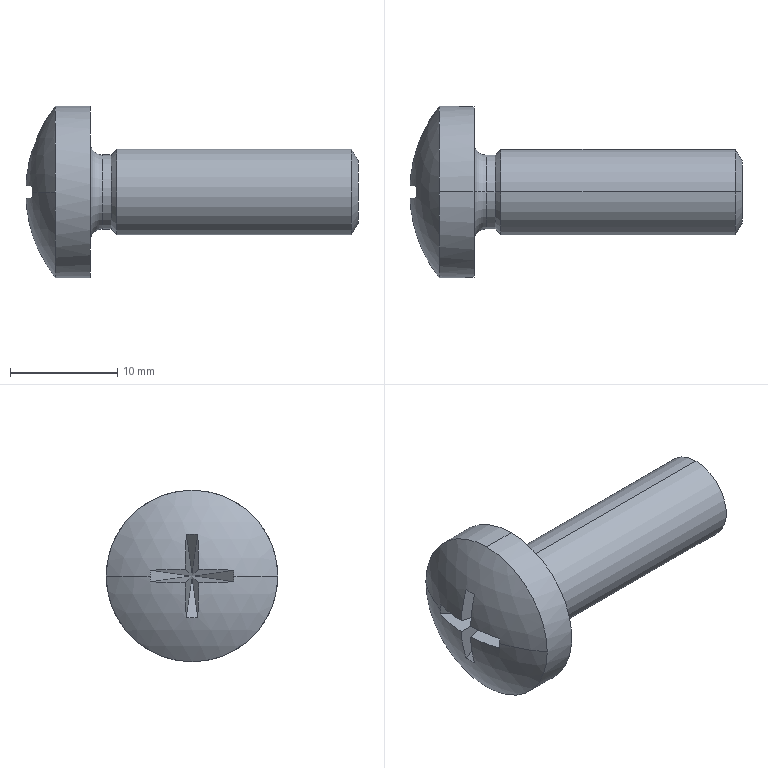Part | SolidWorks | features BlendCut 1, LPattern 1, MirrorPattern 1, RevCut 1, Revolution 1 | 1 solid | 28 faces | box 30.97 x 16 x 16 mm | volume 2140 mm3 | plane 14 | cylinder 6 | cone 4 | torus 2 | sphere 2 | commonest cylinder face diameters 6.928 x2 8 x2 16 x2
STEP:
#1=CARTESIAN_POINT('',(31.,0.,2.918));
#2=VERTEX_POINT('',#1);
#3=CARTESIAN_POINT('',(31.,0.,-2.918));
#4=VERTEX_POINT('',#3);
#5=CARTESIAN_POINT('',(31.,0.,0.));
#6=DIRECTION('',(-1.,0.,0.));
#7=DIRECTION('',(0.,0.,1.));
#8=AXIS2_PLACEMENT_3D('',#5,#6,#7);
#9=CIRCLE('',#8,2.918);
#10=EDGE_CURVE('',#2,#4,#9,.T.);
#11=ORIENTED_EDGE('',*,*,#10,.T.);
#12=CARTESIAN_POINT('',(30.382,0.,-4.));
#13=VERTEX_POINT('',#12);
#14=CARTESIAN_POINT('',(30.382,0.,-4.));
#15=DIRECTION('',(-0.4959,0.,-0.8684));
#16=VECTOR('',#15,1000.);
#17=LINE('',#14,#16);
#18=EDGE_CURVE('',#4,#13,#17,.T.);
#19=ORIENTED_EDGE('',*,*,#18,.T.);
#20=CARTESIAN_POINT('',(30.382,0.,4.));
#21=VERTEX_POINT('',#20);
#22=CARTESIAN_POINT('',(30.382,0.,0.));
#23=DIRECTION('',(-1.,0.,0.));
#24=DIRECTION('',(0.,0.,1.));
#25=AXIS2_PLACEMENT_3D('',#22,#23,#24);
#26=CIRCLE('',#25,4.);
#27=EDGE_CURVE('',#21,#13,#26,.T.);
#28=ORIENTED_EDGE('',*,*,#27,.F.);
#29=CARTESIAN_POINT('',(30.382,0.,4.));
#30=DIRECTION('',(-0.4959,0.,0.8684));
#31=VECTOR('',#30,1000.);
#32=LINE('',#29,#31);
#33=EDGE_CURVE('',#2,#21,#32,.T.);
#34=ORIENTED_EDGE('',*,*,#33,.F.);
#35=EDGE_LOOP('',(#11,#19,#28,#34));
#36=FACE_OUTER_BOUND('',#35,.T.);
#37=CARTESIAN_POINT('',(30.382,0.,0.));
#38=DIRECTION('',(-1.,0.,0.));
#39=DIRECTION('',(0.,0.,1.));
#40=AXIS2_PLACEMENT_3D('',#37,#38,#39);
#41=CONICAL_SURFACE('',#40,4.,1.052);
#42=ADVANCED_FACE('',(#36),#41,.T.);
#43=CARTESIAN_POINT('',(7.964,0.,3.464));
#44=VERTEX_POINT('',#43);
#45=CARTESIAN_POINT('',(7.964,0.,-3.464));
#46=VERTEX_POINT('',#45);
#47=CARTESIAN_POINT('',(7.964,0.,0.));
#48=DIRECTION('',(-1.,0.,0.));
#49=DIRECTION('',(0.,0.,1.));
#50=AXIS2_PLACEMENT_3D('',#47,#48,#49);
#51=CIRCLE('',#50,3.464);
#52=EDGE_CURVE('',#44,#46,#51,.T.);
#53=ORIENTED_EDGE('',*,*,#52,.F.);
#54=CARTESIAN_POINT('',(8.5,0.,4.));
#55=VERTEX_POINT('',#54);
#56=CARTESIAN_POINT('',(8.5,0.,4.));
#57=DIRECTION('',(0.7071,0.,0.7071));
#58=VECTOR('',#57,1000.);
#59=LINE('',#56,#58);
#60=EDGE_CURVE('',#44,#55,#59,.T.);
#61=ORIENTED_EDGE('',*,*,#60,.T.);
#62=CARTESIAN_POINT('',(8.5,0.,-4.));
#63=VERTEX_POINT('',#62);
#64=CARTESIAN_POINT('',(8.5,0.,0.));
#65=DIRECTION('',(-1.,0.,0.));
#66=DIRECTION('',(0.,0.,1.));
#67=AXIS2_PLACEMENT_3D('',#64,#65,#66);
#68=CIRCLE('',#67,4.);
#69=EDGE_CURVE('',#55,#63,#68,.T.);
#70=ORIENTED_EDGE('',*,*,#69,.T.);
#71=CARTESIAN_POINT('',(8.5,0.,-4.));
#72=DIRECTION('',(0.7071,0.,-0.7071));
#73=VECTOR('',#72,1000.);
#74=LINE('',#71,#73);
#75=EDGE_CURVE('',#46,#63,#74,.T.);
#76=ORIENTED_EDGE('',*,*,#75,.F.);
#77=EDGE_LOOP('',(#53,#61,#70,#76));
#78=FACE_OUTER_BOUND('',#77,.T.);
#79=CARTESIAN_POINT('',(8.5,0.,0.));
#80=DIRECTION('',(1.,0.,0.));
#81=DIRECTION('',(0.,0.,-1.));
#82=AXIS2_PLACEMENT_3D('',#79,#80,#81);
#83=CONICAL_SURFACE('',#82,4.,0.7854);
#84=ADVANCED_FACE('',(#78),#83,.T.);
#85=ORIENTED_EDGE('',*,*,#52,.T.);
#86=CARTESIAN_POINT('',(7.136,0.,-3.464));
#87=VERTEX_POINT('',#86);
#88=CARTESIAN_POINT('',(-1.332,0.,-3.464));
#89=DIRECTION('',(-1.,0.,0.));
#90=VECTOR('',#89,1000.);
#91=LINE('',#88,#90);
#92=EDGE_CURVE('',#46,#87,#91,.T.);
#93=ORIENTED_EDGE('',*,*,#92,.T.);
#94=CARTESIAN_POINT('',(7.136,0.,3.464));
#95=VERTEX_POINT('',#94);
#96=CARTESIAN_POINT('',(7.136,0.,0.));
#97=DIRECTION('',(-1.,0.,0.));
#98=DIRECTION('',(0.,0.,1.));
#99=AXIS2_PLACEMENT_3D('',#96,#97,#98);
#100=CIRCLE('',#99,3.464);
#101=EDGE_CURVE('',#95,#87,#100,.T.);
#102=ORIENTED_EDGE('',*,*,#101,.F.);
#103=CARTESIAN_POINT('',(-1.332,0.,3.464));
#104=DIRECTION('',(-1.,0.,0.));
#105=VECTOR('',#104,1000.);
#106=LINE('',#103,#105);
#107=EDGE_CURVE('',#44,#95,#106,.T.);
#108=ORIENTED_EDGE('',*,*,#107,.F.);
#109=EDGE_LOOP('',(#85,#93,#102,#108));
#110=FACE_OUTER_BOUND('',#109,.T.);
#111=CARTESIAN_POINT('',(-1.332,0.,0.));
#112=DIRECTION('',(-1.,0.,0.));
#113=DIRECTION('',(0.,0.,1.));
#114=AXIS2_PLACEMENT_3D('',#111,#112,#113);
#115=CYLINDRICAL_SURFACE('',#114,3.464);
#116=ADVANCED_FACE('',(#110),#115,.T.);
#117=CARTESIAN_POINT('',(6.,0.,-4.6));
#118=VERTEX_POINT('',#117);
#119=CARTESIAN_POINT('',(6.,0.,4.6));
#120=VERTEX_POINT('',#119);
#121=CARTESIAN_POINT('',(6.,0.,0.));
#122=DIRECTION('',(-1.,0.,0.));
#123=DIRECTION('',(0.,0.,1.));
#124=AXIS2_PLACEMENT_3D('',#121,#122,#123);
#125=CIRCLE('',#124,4.6);
#126=EDGE_CURVE('',#118,#120,#125,.T.);
#127=ORIENTED_EDGE('',*,*,#126,.F.);
#128=CARTESIAN_POINT('',(7.136,0.,-4.6));
#129=DIRECTION('',(0.,1.,0.));
#130=DIRECTION('',(0.,0.,1.));
#131=AXIS2_PLACEMENT_3D('',#128,#129,#130);
#132=CIRCLE('',#131,1.136);
#133=EDGE_CURVE('',#118,#87,#132,.T.);
#134=ORIENTED_EDGE('',*,*,#133,.T.);
#135=CARTESIAN_POINT('',(7.136,0.,0.));
#136=DIRECTION('',(-1.,0.,0.));
#137=DIRECTION('',(0.,0.,1.));
#138=AXIS2_PLACEMENT_3D('',#135,#136,#137);
#139=CIRCLE('',#138,3.464);
#140=EDGE_CURVE('',#87,#95,#139,.T.);
#141=ORIENTED_EDGE('',*,*,#140,.T.);
#142=CARTESIAN_POINT('',(7.136,0.,4.6));
#143=DIRECTION('',(0.,-1.,0.));
#144=DIRECTION('',(0.,0.,-1.));
#145=AXIS2_PLACEMENT_3D('',#142,#143,#144);
#146=CIRCLE('',#145,1.136);
#147=EDGE_CURVE('',#120,#95,#146,.T.);
#148=ORIENTED_EDGE('',*,*,#147,.F.);
#149=EDGE_LOOP('',(#127,#134,#141,#148));
#150=FACE_OUTER_BOUND('',#149,.T.);
#151=CARTESIAN_POINT('',(7.136,0.,0.));
#152=DIRECTION('',(-1.,0.,0.));
#153=DIRECTION('',(0.,0.,1.));
#154=AXIS2_PLACEMENT_3D('',#151,#152,#153);
#155=TOROIDAL_SURFACE('',#154,4.6,1.136);
#156=ADVANCED_FACE('',(#150),#155,.F.);
#157=CARTESIAN_POINT('',(6.,0.,8.));
#158=VERTEX_POINT('',#157);
#159=CARTESIAN_POINT('',(6.,0.,-8.));
#160=VERTEX_POINT('',#159);
#161=CARTESIAN_POINT('',(6.,0.,0.));
#162=DIRECTION('',(-1.,0.,0.));
#163=DIRECTION('',(0.,0.,1.));
#164=AXIS2_PLACEMENT_3D('',#161,#162,#163);
#165=CIRCLE('',#164,8.);
#166=EDGE_CURVE('',#158,#160,#165,.T.);
#167=ORIENTED_EDGE('',*,*,#166,.T.);
#168=CARTESIAN_POINT('',(2.753,0.,-8.));
#169=VERTEX_POINT('',#168);
#170=CARTESIAN_POINT('',(-1.332,0.,-8.));
#171=DIRECTION('',(-1.,0.,0.));
#172=VECTOR('',#171,1000.);
#173=LINE('',#170,#172);
#174=EDGE_CURVE('',#160,#169,#173,.T.);
#175=ORIENTED_EDGE('',*,*,#174,.T.);
#176=CARTESIAN_POINT('',(2.753,8.,0.));
#177=VERTEX_POINT('',#176);
#178=CARTESIAN_POINT('',(2.753,0.,0.));
#179=DIRECTION('',(-1.,0.,0.));
#180=DIRECTION('',(0.,0.,1.));
#181=AXIS2_PLACEMENT_3D('',#178,#179,#180);
#182=CIRCLE('',#181,8.);
#183=EDGE_CURVE('',#177,#169,#182,.T.);
#184=ORIENTED_EDGE('',*,*,#183,.F.);
#185=CARTESIAN_POINT('',(2.753,0.,8.));
#186=VERTEX_POINT('',#185);
#187=CARTESIAN_POINT('',(2.753,0.,0.));
#188=DIRECTION('',(-1.,0.,0.));
#189=DIRECTION('',(0.,0.,1.));
#190=AXIS2_PLACEMENT_3D('',#187,#188,#189);
#191=CIRCLE('',#190,8.);
#192=EDGE_CURVE('',#186,#177,#191,.T.);
#193=ORIENTED_EDGE('',*,*,#192,.F.);
#194=CARTESIAN_POINT('',(-1.332,0.,8.));
#195=DIRECTION('',(-1.,0.,0.));
#196=VECTOR('',#195,1000.);
#197=LINE('',#194,#196);
#198=EDGE_CURVE('',#158,#186,#197,.T.);
#199=ORIENTED_EDGE('',*,*,#198,.F.);
#200=EDGE_LOOP('',(#167,#175,#184,#193,#199));
#201=FACE_OUTER_BOUND('',#200,.T.);
#202=CARTESIAN_POINT('',(-1.332,0.,0.));
#203=DIRECTION('',(-1.,0.,0.));
#204=DIRECTION('',(0.,0.,1.));
#205=AXIS2_PLACEMENT_3D('',#202,#203,#204);
#206=CYLINDRICAL_SURFACE('',#205,8.);
#207=ADVANCED_FACE('',(#201),#206,.T.);
#208=ORIENTED_EDGE('',*,*,#183,.T.);
#209=CARTESIAN_POINT('',(2.753,-8.,0.));
#210=VERTEX_POINT('',#209);
#211=CARTESIAN_POINT('',(2.753,0.,0.));
#212=DIRECTION('',(-1.,0.,0.));
#213=DIRECTION('',(0.,0.,1.));
#214=AXIS2_PLACEMENT_3D('',#211,#212,#213);
#215=CIRCLE('',#214,8.);
#216=EDGE_CURVE('',#169,#210,#215,.T.);
#217=ORIENTED_EDGE('',*,*,#216,.T.);
#218=CARTESIAN_POINT('',(0.6022,-3.911,0.));
#219=VERTEX_POINT('',#218);
#220=CARTESIAN_POINT('',(13.,0.,0.));
#221=DIRECTION('',(0.,0.,-1.));
#222=DIRECTION('',(0.,1.,0.));
#223=AXIS2_PLACEMENT_3D('',#220,#221,#222);
#224=CIRCLE('',#223,13.);
#225=EDGE_CURVE('',#210,#219,#224,.T.);
#226=ORIENTED_EDGE('',*,*,#225,.T.);
#227=CARTESIAN_POINT('',(0.6113,-3.902,-0.5419));
#228=VERTEX_POINT('',#227);
#229=CARTESIAN_POINT('',(8.892,4.199,0.));
#230=DIRECTION('',(0.6993,-0.7148,0.));
#231=DIRECTION('',(0.7148,0.6993,0.));
#232=AXIS2_PLACEMENT_3D('',#229,#230,#231);
#233=CIRCLE('',#232,11.597);
#234=EDGE_CURVE('',#219,#228,#233,.T.);
#235=ORIENTED_EDGE('',*,*,#234,.T.);
#236=CARTESIAN_POINT('',(0.0297,-0.621,-0.621));
#237=VERTEX_POINT('',#236);
#238=CARTESIAN_POINT('',(12.848,0.,1.121));
#239=DIRECTION('',(0.1346,0.,-0.9909));
#240=DIRECTION('',(-0.9909,0.,-0.1346));
#241=AXIS2_PLACEMENT_3D('',#238,#239,#240);
#242=CIRCLE('',#241,12.951);
#243=EDGE_CURVE('',#228,#237,#242,.T.);
#244=ORIENTED_EDGE('',*,*,#243,.T.);
#245=CARTESIAN_POINT('',(0.6113,-0.5419,-3.902));
#246=VERTEX_POINT('',#245);
#247=CARTESIAN_POINT('',(12.848,1.121,0.));
#248=DIRECTION('',(0.1346,-0.9909,0.));
#249=DIRECTION('',(0.9909,0.1346,0.));
#250=AXIS2_PLACEMENT_3D('',#247,#248,#249);
#251=CIRCLE('',#250,12.951);
#252=EDGE_CURVE('',#237,#246,#251,.T.);
#253=ORIENTED_EDGE('',*,*,#252,.T.);
#254=CARTESIAN_POINT('',(0.6113,0.5419,-3.902));
#255=VERTEX_POINT('',#254);
#256=CARTESIAN_POINT('',(8.892,0.,4.199));
#257=DIRECTION('',(0.6993,0.,-0.7148));
#258=DIRECTION('',(-0.7148,0.,-0.6993));
#259=AXIS2_PLACEMENT_3D('',#256,#257,#258);
#260=CIRCLE('',#259,11.597);
#261=EDGE_CURVE('',#246,#255,#260,.T.);
#262=ORIENTED_EDGE('',*,*,#261,.T.);
#263=CARTESIAN_POINT('',(0.0297,0.621,-0.621));
#264=VERTEX_POINT('',#263);
#265=CARTESIAN_POINT('',(12.848,-1.121,0.));
#266=DIRECTION('',(0.1346,0.9909,0.));
#267=DIRECTION('',(-0.9909,0.1346,0.));
#268=AXIS2_PLACEMENT_3D('',#265,#266,#267);
#269=CIRCLE('',#268,12.951);
#270=EDGE_CURVE('',#255,#264,#269,.T.);
#271=ORIENTED_EDGE('',*,*,#270,.T.);
#272=CARTESIAN_POINT('',(0.6113,3.902,-0.5419));
#273=VERTEX_POINT('',#272);
#274=CARTESIAN_POINT('',(12.848,0.,1.121));
#275=DIRECTION('',(0.1346,0.,-0.9909));
#276=DIRECTION('',(-0.9909,0.,-0.1346));
#277=AXIS2_PLACEMENT_3D('',#274,#275,#276);
#278=CIRCLE('',#277,12.951);
#279=EDGE_CURVE('',#264,#273,#278,.T.);
#280=ORIENTED_EDGE('',*,*,#279,.T.);
#281=CARTESIAN_POINT('',(0.6022,3.911,0.));
#282=VERTEX_POINT('',#281);
#283=CARTESIAN_POINT('',(8.892,-4.199,0.));
#284=DIRECTION('',(0.6993,0.7148,0.));
#285=DIRECTION('',(-0.7148,0.6993,0.));
#286=AXIS2_PLACEMENT_3D('',#283,#284,#285);
#287=CIRCLE('',#286,11.597);
#288=EDGE_CURVE('',#273,#282,#287,.T.);
#289=ORIENTED_EDGE('',*,*,#288,.T.);
#290=CARTESIAN_POINT('',(13.,0.,0.));
#291=DIRECTION('',(0.,0.,1.));
#292=DIRECTION('',(1.,0.,0.));
#293=AXIS2_PLACEMENT_3D('',#290,#291,#292);
#294=CIRCLE('',#293,13.);
#295=EDGE_CURVE('',#177,#282,#294,.T.);
#296=ORIENTED_EDGE('',*,*,#295,.F.);
#297=EDGE_LOOP('',(#208,#217,#226,#235,#244,#253,#262,#271,#280,#289,#296));
#298=FACE_OUTER_BOUND('',#297,.T.);
#299=CARTESIAN_POINT('',(13.,0.,0.));
#300=DIRECTION('',(0.,0.,-1.));
#301=DIRECTION('',(0.,1.,0.));
#302=AXIS2_PLACEMENT_3D('',#299,#300,#301);
#303=SPHERICAL_SURFACE('',#302,13.);
#304=ADVANCED_FACE('',(#298),#303,.T.);
#305=ORIENTED_EDGE('',*,*,#27,.T.);
#306=CARTESIAN_POINT('',(-1.332,0.,-4.));
#307=DIRECTION('',(-1.,0.,0.));
#308=VECTOR('',#307,1000.);
#309=LINE('',#306,#308);
#310=EDGE_CURVE('',#13,#63,#309,.T.);
#311=ORIENTED_EDGE('',*,*,#310,.T.);
#312=ORIENTED_EDGE('',*,*,#69,.F.);
#313=CARTESIAN_POINT('',(-1.332,0.,4.));
#314=DIRECTION('',(-1.,0.,0.));
#315=VECTOR('',#314,1000.);
#316=LINE('',#313,#315);
#317=EDGE_CURVE('',#21,#55,#316,.T.);
#318=ORIENTED_EDGE('',*,*,#317,.F.);
#319=EDGE_LOOP('',(#305,#311,#312,#318));
#320=FACE_OUTER_BOUND('',#319,.T.);
#321=CARTESIAN_POINT('',(-1.332,0.,0.));
#322=DIRECTION('',(-1.,0.,0.));
#323=DIRECTION('',(0.,0.,1.));
#324=AXIS2_PLACEMENT_3D('',#321,#322,#323);
#325=CYLINDRICAL_SURFACE('',#324,4.);
#326=ADVANCED_FACE('',(#320),#325,.T.);
#327=CARTESIAN_POINT('',(4.6,0.,0.));
#328=VERTEX_POINT('',#327);
#329=CARTESIAN_POINT('',(4.6,0.,0.));
#330=DIRECTION('',(-0.7115,-0.696,-0.09667));
#331=VECTOR('',#330,1000.);
#332=LINE('',#329,#331);
#333=EDGE_CURVE('',#328,#228,#332,.T.);
#334=ORIENTED_EDGE('',*,*,#333,.F.);
#335=CARTESIAN_POINT('',(4.6,0.,0.));
#336=DIRECTION('',(-0.982,-0.1334,-0.1334));
#337=VECTOR('',#336,1000.);
#338=LINE('',#335,#337);
#339=EDGE_CURVE('',#328,#237,#338,.T.);
#340=ORIENTED_EDGE('',*,*,#339,.T.);
#341=ORIENTED_EDGE('',*,*,#243,.F.);
#342=EDGE_LOOP('',(#334,#340,#341));
#343=FACE_OUTER_BOUND('',#342,.T.);
#344=CARTESIAN_POINT('',(4.6,0.,0.));
#345=DIRECTION('',(0.1346,0.,-0.9909));
#346=DIRECTION('',(-0.9909,0.,-0.1346));
#347=AXIS2_PLACEMENT_3D('',#344,#345,#346);
#348=PLANE('',#347);
#349=ADVANCED_FACE('',(#343),#348,.F.);
#350=CARTESIAN_POINT('',(0.0297,-0.621,0.621));
#351=VERTEX_POINT('',#350);
#352=CARTESIAN_POINT('',(0.6113,-3.902,0.5419));
#353=VERTEX_POINT('',#352);
#354=CARTESIAN_POINT('',(12.848,0.,-1.121));
#355=DIRECTION('',(0.1346,0.,0.9909));
#356=DIRECTION('',(0.9909,0.,-0.1346));
#357=AXIS2_PLACEMENT_3D('',#354,#355,#356);
#358=CIRCLE('',#357,12.951);
#359=EDGE_CURVE('',#351,#353,#358,.T.);
#360=ORIENTED_EDGE('',*,*,#359,.F.);
#361=CARTESIAN_POINT('',(4.6,0.,0.));
#362=DIRECTION('',(0.982,0.1334,-0.1334));
#363=VECTOR('',#362,1000.);
#364=LINE('',#361,#363);
#365=EDGE_CURVE('',#351,#328,#364,.T.);
#366=ORIENTED_EDGE('',*,*,#365,.T.);
#367=CARTESIAN_POINT('',(4.6,0.,0.));
#368=DIRECTION('',(-0.7115,-0.696,0.09667));
#369=VECTOR('',#368,1000.);
#370=LINE('',#367,#369);
#371=EDGE_CURVE('',#328,#353,#370,.T.);
#372=ORIENTED_EDGE('',*,*,#371,.T.);
#373=EDGE_LOOP('',(#360,#366,#372));
#374=FACE_OUTER_BOUND('',#373,.T.);
#375=CARTESIAN_POINT('',(4.6,0.,0.));
#376=DIRECTION('',(0.1346,0.,0.9909));
#377=DIRECTION('',(0.9909,0.,-0.1346));
#378=AXIS2_PLACEMENT_3D('',#375,#376,#377);
#379=PLANE('',#378);
#380=ADVANCED_FACE('',(#374),#379,.F.);
#381=ORIENTED_EDGE('',*,*,#310,.F.);
#382=CARTESIAN_POINT('',(30.382,0.,0.));
#383=DIRECTION('',(-1.,0.,0.));
#384=DIRECTION('',(0.,0.,1.));
#385=AXIS2_PLACEMENT_3D('',#382,#383,#384);
#386=CIRCLE('',#385,4.);
#387=EDGE_CURVE('',#13,#21,#386,.T.);
#388=ORIENTED_EDGE('',*,*,#387,.T.);
#389=ORIENTED_EDGE('',*,*,#317,.T.);
#390=CARTESIAN_POINT('',(8.5,0.,0.));
#391=DIRECTION('',(-1.,0.,0.));
#392=DIRECTION('',(0.,0.,1.));
#393=AXIS2_PLACEMENT_3D('',#390,#391,#392);
#394=CIRCLE('',#393,4.);
#395=EDGE_CURVE('',#63,#55,#394,.T.);
#396=ORIENTED_EDGE('',*,*,#395,.F.);
#397=EDGE_LOOP('',(#381,#388,#389,#396));
#398=FACE_OUTER_BOUND('',#397,.T.);
#399=CARTESIAN_POINT('',(-1.332,0.,0.));
#400=DIRECTION('',(-1.,0.,0.));
#401=DIRECTION('',(0.,0.,1.));
#402=AXIS2_PLACEMENT_3D('',#399,#400,#401);
#403=CYLINDRICAL_SURFACE('',#402,4.);
#404=ADVANCED_FACE('',(#398),#403,.T.);
#405=ORIENTED_EDGE('',*,*,#225,.F.);
#406=CARTESIAN_POINT('',(2.753,0.,0.));
#407=DIRECTION('',(-1.,0.,0.));
#408=DIRECTION('',(0.,0.,1.));
#409=AXIS2_PLACEMENT_3D('',#406,#407,#408);
#410=CIRCLE('',#409,8.);
#411=EDGE_CURVE('',#210,#186,#410,.T.);
#412=ORIENTED_EDGE('',*,*,#411,.T.);
#413=ORIENTED_EDGE('',*,*,#192,.T.);
#414=ORIENTED_EDGE('',*,*,#295,.T.);
#415=CARTESIAN_POINT('',(0.6113,3.902,0.5419));
#416=VERTEX_POINT('',#415);
#417=CARTESIAN_POINT('',(8.892,-4.199,0.));
#418=DIRECTION('',(0.6993,0.7148,0.));
#419=DIRECTION('',(-0.7148,0.6993,0.));
#420=AXIS2_PLACEMENT_3D('',#417,#418,#419);
#421=CIRCLE('',#420,11.597);
#422=EDGE_CURVE('',#282,#416,#421,.T.);
#423=ORIENTED_EDGE('',*,*,#422,.T.);
#424=CARTESIAN_POINT('',(0.0297,0.621,0.621));
#425=VERTEX_POINT('',#424);
#426=CARTESIAN_POINT('',(12.848,0.,-1.121));
#427=DIRECTION('',(0.1346,0.,0.9909));
#428=DIRECTION('',(0.9909,0.,-0.1346));
#429=AXIS2_PLACEMENT_3D('',#426,#427,#428);
#430=CIRCLE('',#429,12.951);
#431=EDGE_CURVE('',#416,#425,#430,.T.);
#432=ORIENTED_EDGE('',*,*,#431,.T.);
#433=CARTESIAN_POINT('',(0.6113,0.5419,3.902));
#434=VERTEX_POINT('',#433);
#435=CARTESIAN_POINT('',(12.848,-1.121,0.));
#436=DIRECTION('',(0.1346,0.9909,0.));
#437=DIRECTION('',(-0.9909,0.1346,0.));
#438=AXIS2_PLACEMENT_3D('',#435,#436,#437);
#439=CIRCLE('',#438,12.951);
#440=EDGE_CURVE('',#425,#434,#439,.T.);
#441=ORIENTED_EDGE('',*,*,#440,.T.);
#442=CARTESIAN_POINT('',(0.6113,-0.5419,3.902));
#443=VERTEX_POINT('',#442);
#444=CARTESIAN_POINT('',(8.892,0.,-4.199));
#445=DIRECTION('',(0.6993,0.,0.7148));
#446=DIRECTION('',(0.7148,0.,-0.6993));
#447=AXIS2_PLACEMENT_3D('',#444,#445,#446);
#448=CIRCLE('',#447,11.597);
#449=EDGE_CURVE('',#434,#443,#448,.T.);
#450=ORIENTED_EDGE('',*,*,#449,.T.);
#451=CARTESIAN_POINT('',(12.848,1.121,0.));
#452=DIRECTION('',(0.1346,-0.9909,0.));
#453=DIRECTION('',(0.9909,0.1346,0.));
#454=AXIS2_PLACEMENT_3D('',#451,#452,#453);
#455=CIRCLE('',#454,12.951);
#456=EDGE_CURVE('',#443,#351,#455,.T.);
#457=ORIENTED_EDGE('',*,*,#456,.T.);
#458=ORIENTED_EDGE('',*,*,#359,.T.);
#459=CARTESIAN_POINT('',(8.892,4.199,0.));
#460=DIRECTION('',(0.6993,-0.7148,0.));
#461=DIRECTION('',(0.7148,0.6993,0.));
#462=AXIS2_PLACEMENT_3D('',#459,#460,#461);
#463=CIRCLE('',#462,11.597);
#464=EDGE_CURVE('',#353,#219,#463,.T.);
#465=ORIENTED_EDGE('',*,*,#464,.T.);
#466=EDGE_LOOP('',(#405,#412,#413,#414,#423,#432,#441,#450,#457,#458,#465));
#467=FACE_OUTER_BOUND('',#466,.T.);
#468=CARTESIAN_POINT('',(13.,0.,0.));
#469=DIRECTION('',(0.,0.,-1.));
#470=DIRECTION('',(0.,1.,0.));
#471=AXIS2_PLACEMENT_3D('',#468,#469,#470);
#472=SPHERICAL_SURFACE('',#471,13.);
#473=ADVANCED_FACE('',(#467),#472,.T.);
#474=ORIENTED_EDGE('',*,*,#174,.F.);
#475=CARTESIAN_POINT('',(6.,0.,0.));
#476=DIRECTION('',(-1.,0.,0.));
#477=DIRECTION('',(0.,0.,1.));
#478=AXIS2_PLACEMENT_3D('',#475,#476,#477);
#479=CIRCLE('',#478,8.);
#480=EDGE_CURVE('',#160,#158,#479,.T.);
#481=ORIENTED_EDGE('',*,*,#480,.T.);
#482=ORIENTED_EDGE('',*,*,#198,.T.);
#483=ORIENTED_EDGE('',*,*,#411,.F.);
#484=ORIENTED_EDGE('',*,*,#216,.F.);
#485=EDGE_LOOP('',(#474,#481,#482,#483,#484));
#486=FACE_OUTER_BOUND('',#485,.T.);
#487=CARTESIAN_POINT('',(-1.332,0.,0.));
#488=DIRECTION('',(-1.,0.,0.));
#489=DIRECTION('',(0.,0.,1.));
#490=AXIS2_PLACEMENT_3D('',#487,#488,#489);
#491=CYLINDRICAL_SURFACE('',#490,8.);
#492=ADVANCED_FACE('',(#486),#491,.T.);
#493=ORIENTED_EDGE('',*,*,#166,.F.);
#494=ORIENTED_EDGE('',*,*,#480,.F.);
#495=EDGE_LOOP('',(#493,#494));
#496=FACE_OUTER_BOUND('',#495,.T.);
#497=CARTESIAN_POINT('',(6.,0.,0.));
#498=DIRECTION('',(-1.,0.,0.));
#499=DIRECTION('',(0.,0.,1.));
#500=AXIS2_PLACEMENT_3D('',#497,#498,#499);
#501=CIRCLE('',#500,4.6);
#502=EDGE_CURVE('',#120,#118,#501,.T.);
#503=ORIENTED_EDGE('',*,*,#502,.T.);
#504=ORIENTED_EDGE('',*,*,#126,.T.);
#505=EDGE_LOOP('',(#503,#504));
#506=FACE_BOUND('',#505,.T.);
#507=CARTESIAN_POINT('',(6.,4.6,0.));
#508=DIRECTION('',(-1.,0.,0.));
#509=DIRECTION('',(0.,0.,1.));
#510=AXIS2_PLACEMENT_3D('',#507,#508,#509);
#511=PLANE('',#510);
#512=ADVANCED_FACE('',(#496,#506),#511,.F.);
#513=ORIENTED_EDGE('',*,*,#133,.F.);
#514=ORIENTED_EDGE('',*,*,#502,.F.);
#515=ORIENTED_EDGE('',*,*,#147,.T.);
#516=ORIENTED_EDGE('',*,*,#101,.T.);
#517=EDGE_LOOP('',(#513,#514,#515,#516));
#518=FACE_OUTER_BOUND('',#517,.T.);
#519=CARTESIAN_POINT('',(7.136,0.,0.));
#520=DIRECTION('',(-1.,0.,0.));
#521=DIRECTION('',(0.,0.,1.));
#522=AXIS2_PLACEMENT_3D('',#519,#520,#521);
#523=TOROIDAL_SURFACE('',#522,4.6,1.136);
#524=ADVANCED_FACE('',(#518),#523,.F.);
#525=ORIENTED_EDGE('',*,*,#92,.F.);
#526=CARTESIAN_POINT('',(7.964,0.,0.));
#527=DIRECTION('',(-1.,0.,0.));
#528=DIRECTION('',(0.,0.,1.));
#529=AXIS2_PLACEMENT_3D('',#526,#527,#528);
#530=CIRCLE('',#529,3.464);
#531=EDGE_CURVE('',#46,#44,#530,.T.);
#532=ORIENTED_EDGE('',*,*,#531,.T.);
#533=ORIENTED_EDGE('',*,*,#107,.T.);
#534=ORIENTED_EDGE('',*,*,#140,.F.);
#535=EDGE_LOOP('',(#525,#532,#533,#534));
#536=FACE_OUTER_BOUND('',#535,.T.);
#537=CARTESIAN_POINT('',(-1.332,0.,0.));
#538=DIRECTION('',(-1.,0.,0.));
#539=DIRECTION('',(0.,0.,1.));
#540=AXIS2_PLACEMENT_3D('',#537,#538,#539);
#541=CYLINDRICAL_SURFACE('',#540,3.464);
#542=ADVANCED_FACE('',(#536),#541,.T.);
#543=ORIENTED_EDGE('',*,*,#60,.F.);
#544=ORIENTED_EDGE('',*,*,#531,.F.);
#545=ORIENTED_EDGE('',*,*,#75,.T.);
#546=ORIENTED_EDGE('',*,*,#395,.T.);
#547=EDGE_LOOP('',(#543,#544,#545,#546));
#548=FACE_OUTER_BOUND('',#547,.T.);
#549=CARTESIAN_POINT('',(8.5,0.,0.));
#550=DIRECTION('',(1.,0.,0.));
#551=DIRECTION('',(0.,0.,-1.));
#552=AXIS2_PLACEMENT_3D('',#549,#550,#551);
#553=CONICAL_SURFACE('',#552,4.,0.7854);
#554=ADVANCED_FACE('',(#548),#553,.T.);
#555=ORIENTED_EDGE('',*,*,#18,.F.);
#556=CARTESIAN_POINT('',(31.,0.,0.));
#557=DIRECTION('',(-1.,0.,0.));
#558=DIRECTION('',(0.,0.,1.));
#559=AXIS2_PLACEMENT_3D('',#556,#557,#558);
#560=CIRCLE('',#559,2.918);
#561=EDGE_CURVE('',#4,#2,#560,.T.);
#562=ORIENTED_EDGE('',*,*,#561,.T.);
#563=ORIENTED_EDGE('',*,*,#33,.T.);
#564=ORIENTED_EDGE('',*,*,#387,.F.);
#565=EDGE_LOOP('',(#555,#562,#563,#564));
#566=FACE_OUTER_BOUND('',#565,.T.);
#567=CARTESIAN_POINT('',(30.382,0.,0.));
#568=DIRECTION('',(-1.,0.,0.));
#569=DIRECTION('',(0.,0.,1.));
#570=AXIS2_PLACEMENT_3D('',#567,#568,#569);
#571=CONICAL_SURFACE('',#570,4.,1.052);
#572=ADVANCED_FACE('',(#566),#571,.T.);
#573=ORIENTED_EDGE('',*,*,#10,.F.);
#574=ORIENTED_EDGE('',*,*,#561,.F.);
#575=EDGE_LOOP('',(#573,#574));
#576=FACE_OUTER_BOUND('',#575,.T.);
#577=CARTESIAN_POINT('',(31.,0.,0.));
#578=DIRECTION('',(-1.,0.,0.));
#579=DIRECTION('',(0.,0.,1.));
#580=AXIS2_PLACEMENT_3D('',#577,#578,#579);
#581=PLANE('',#580);
#582=ADVANCED_FACE('',(#576),#581,.F.);
#583=ORIENTED_EDGE('',*,*,#279,.F.);
#584=CARTESIAN_POINT('',(4.6,0.,0.));
#585=DIRECTION('',(0.982,-0.1334,0.1334));
#586=VECTOR('',#585,1000.);
#587=LINE('',#584,#586);
#588=EDGE_CURVE('',#264,#328,#587,.T.);
#589=ORIENTED_EDGE('',*,*,#588,.T.);
#590=CARTESIAN_POINT('',(4.6,0.,0.));
#591=DIRECTION('',(-0.7115,0.696,-0.09667));
#592=VECTOR('',#591,1000.);
#593=LINE('',#590,#592);
#594=EDGE_CURVE('',#328,#273,#593,.T.);
#595=ORIENTED_EDGE('',*,*,#594,.T.);
#596=EDGE_LOOP('',(#583,#589,#595));
#597=FACE_OUTER_BOUND('',#596,.T.);
#598=CARTESIAN_POINT('',(4.6,0.,0.));
#599=DIRECTION('',(0.1346,0.,-0.9909));
#600=DIRECTION('',(-0.9909,0.,-0.1346));
#601=AXIS2_PLACEMENT_3D('',#598,#599,#600);
#602=PLANE('',#601);
#603=ADVANCED_FACE('',(#597),#602,.F.);
#604=ORIENTED_EDGE('',*,*,#594,.F.);
#605=CARTESIAN_POINT('',(4.6,0.,0.));
#606=DIRECTION('',(-0.7115,0.696,0.09667));
#607=VECTOR('',#606,1000.);
#608=LINE('',#605,#607);
#609=EDGE_CURVE('',#328,#416,#608,.T.);
#610=ORIENTED_EDGE('',*,*,#609,.T.);
#611=ORIENTED_EDGE('',*,*,#422,.F.);
#612=ORIENTED_EDGE('',*,*,#288,.F.);
#613=EDGE_LOOP('',(#604,#610,#611,#612));
#614=FACE_OUTER_BOUND('',#613,.T.);
#615=CARTESIAN_POINT('',(0.,4.5,-0.625));
#616=DIRECTION('',(0.6993,0.7148,0.));
#617=DIRECTION('',(-0.7148,0.6993,0.));
#618=AXIS2_PLACEMENT_3D('',#615,#616,#617);
#619=PLANE('',#618);
#620=ADVANCED_FACE('',(#614),#619,.F.);
#621=ORIENTED_EDGE('',*,*,#371,.F.);
#622=ORIENTED_EDGE('',*,*,#333,.T.);
#623=ORIENTED_EDGE('',*,*,#234,.F.);
#624=ORIENTED_EDGE('',*,*,#464,.F.);
#625=EDGE_LOOP('',(#621,#622,#623,#624));
#626=FACE_OUTER_BOUND('',#625,.T.);
#627=CARTESIAN_POINT('',(0.,-4.5,0.625));
#628=DIRECTION('',(0.6993,-0.7148,0.));
#629=DIRECTION('',(0.7148,0.6993,0.));
#630=AXIS2_PLACEMENT_3D('',#627,#628,#629);
#631=PLANE('',#630);
#632=ADVANCED_FACE('',(#626),#631,.F.);
#633=ORIENTED_EDGE('',*,*,#609,.F.);
#634=CARTESIAN_POINT('',(4.6,0.,0.));
#635=DIRECTION('',(-0.982,0.1334,0.1334));
#636=VECTOR('',#635,1000.);
#637=LINE('',#634,#636);
#638=EDGE_CURVE('',#328,#425,#637,.T.);
#639=ORIENTED_EDGE('',*,*,#638,.T.);
#640=ORIENTED_EDGE('',*,*,#431,.F.);
#641=EDGE_LOOP('',(#633,#639,#640));
#642=FACE_OUTER_BOUND('',#641,.T.);
#643=CARTESIAN_POINT('',(4.6,0.,0.));
#644=DIRECTION('',(0.1346,0.,0.9909));
#645=DIRECTION('',(0.9909,0.,-0.1346));
#646=AXIS2_PLACEMENT_3D('',#643,#644,#645);
#647=PLANE('',#646);
#648=ADVANCED_FACE('',(#642),#647,.F.);
#649=CARTESIAN_POINT('',(4.6,0.,0.));
#650=DIRECTION('',(-0.7115,-0.09667,0.696));
#651=VECTOR('',#650,1000.);
#652=LINE('',#649,#651);
#653=EDGE_CURVE('',#328,#443,#652,.T.);
#654=ORIENTED_EDGE('',*,*,#653,.F.);
#655=ORIENTED_EDGE('',*,*,#365,.F.);
#656=ORIENTED_EDGE('',*,*,#456,.F.);
#657=EDGE_LOOP('',(#654,#655,#656));
#658=FACE_OUTER_BOUND('',#657,.T.);
#659=CARTESIAN_POINT('',(4.6,0.,0.));
#660=DIRECTION('',(0.1346,-0.9909,0.));
#661=DIRECTION('',(-0.9909,-0.1346,0.));
#662=AXIS2_PLACEMENT_3D('',#659,#660,#661);
#663=PLANE('',#662);
#664=ADVANCED_FACE('',(#658),#663,.F.);
#665=ORIENTED_EDGE('',*,*,#638,.F.);
#666=CARTESIAN_POINT('',(4.6,0.,0.));
#667=DIRECTION('',(-0.7115,0.09667,0.696));
#668=VECTOR('',#667,1000.);
#669=LINE('',#666,#668);
#670=EDGE_CURVE('',#328,#434,#669,.T.);
#671=ORIENTED_EDGE('',*,*,#670,.T.);
#672=ORIENTED_EDGE('',*,*,#440,.F.);
#673=EDGE_LOOP('',(#665,#671,#672));
#674=FACE_OUTER_BOUND('',#673,.T.);
#675=CARTESIAN_POINT('',(4.6,0.,0.));
#676=DIRECTION('',(0.1346,0.9909,0.));
#677=DIRECTION('',(0.9909,-0.1346,0.));
#678=AXIS2_PLACEMENT_3D('',#675,#676,#677);
#679=PLANE('',#678);
#680=ADVANCED_FACE('',(#674),#679,.F.);
#681=ORIENTED_EDGE('',*,*,#670,.F.);
#682=ORIENTED_EDGE('',*,*,#653,.T.);
#683=ORIENTED_EDGE('',*,*,#449,.F.);
#684=EDGE_LOOP('',(#681,#682,#683));
#685=FACE_OUTER_BOUND('',#684,.T.);
#686=CARTESIAN_POINT('',(0.,-0.625,4.5));
#687=DIRECTION('',(0.6993,0.,0.7148));
#688=DIRECTION('',(-0.7148,0.,0.6993));
#689=AXIS2_PLACEMENT_3D('',#686,#687,#688);
#690=PLANE('',#689);
#691=ADVANCED_FACE('',(#685),#690,.F.);
#692=ORIENTED_EDGE('',*,*,#339,.F.);
#693=CARTESIAN_POINT('',(4.6,0.,0.));
#694=DIRECTION('',(-0.7115,-0.09667,-0.696));
#695=VECTOR('',#694,1000.);
#696=LINE('',#693,#695);
#697=EDGE_CURVE('',#328,#246,#696,.T.);
#698=ORIENTED_EDGE('',*,*,#697,.T.);
#699=ORIENTED_EDGE('',*,*,#252,.F.);
#700=EDGE_LOOP('',(#692,#698,#699));
#701=FACE_OUTER_BOUND('',#700,.T.);
#702=CARTESIAN_POINT('',(4.6,0.,0.));
#703=DIRECTION('',(0.1346,-0.9909,0.));
#704=DIRECTION('',(-0.9909,-0.1346,0.));
#705=AXIS2_PLACEMENT_3D('',#702,#703,#704);
#706=PLANE('',#705);
#707=ADVANCED_FACE('',(#701),#706,.F.);
#708=ORIENTED_EDGE('',*,*,#697,.F.);
#709=CARTESIAN_POINT('',(4.6,0.,0.));
#710=DIRECTION('',(-0.7115,0.09667,-0.696));
#711=VECTOR('',#710,1000.);
#712=LINE('',#709,#711);
#713=EDGE_CURVE('',#328,#255,#712,.T.);
#714=ORIENTED_EDGE('',*,*,#713,.T.);
#715=ORIENTED_EDGE('',*,*,#261,.F.);
#716=EDGE_LOOP('',(#708,#714,#715));
#717=FACE_OUTER_BOUND('',#716,.T.);
#718=CARTESIAN_POINT('',(0.,0.625,-4.5));
#719=DIRECTION('',(0.6993,0.,-0.7148));
#720=DIRECTION('',(0.7148,0.,0.6993));
#721=AXIS2_PLACEMENT_3D('',#718,#719,#720);
#722=PLANE('',#721);
#723=ADVANCED_FACE('',(#717),#722,.F.);
#724=ORIENTED_EDGE('',*,*,#713,.F.);
#725=ORIENTED_EDGE('',*,*,#588,.F.);
#726=ORIENTED_EDGE('',*,*,#270,.F.);
#727=EDGE_LOOP('',(#724,#725,#726));
#728=FACE_OUTER_BOUND('',#727,.T.);
#729=CARTESIAN_POINT('',(4.6,0.,0.));
#730=DIRECTION('',(0.1346,0.9909,0.));
#731=DIRECTION('',(0.9909,-0.1346,0.));
#732=AXIS2_PLACEMENT_3D('',#729,#730,#731);
#733=PLANE('',#732);
#734=ADVANCED_FACE('',(#728),#733,.F.);
#735=CLOSED_SHELL('',(#42,#84,#116,#156,#207,#304,#326,#349,#380,#404,#473,#492,#512,#524,#542,#554,#572,#582,#603,#620,#632,#648,#664,#680,#691,#707,#723,#734));
#736=MANIFOLD_SOLID_BREP('',#735);
#737=CARTESIAN_POINT('',(0.,0.,0.));
#738=DIRECTION('',(0.,0.,1.));
#739=DIRECTION('',(1.,0.,0.));
#740=AXIS2_PLACEMENT_3D('',#737,#738,#739);
#741=(LENGTH_UNIT()NAMED_UNIT(*)SI_UNIT(.MILLI.,.METRE.));
#742=UNCERTAINTY_MEASURE_WITH_UNIT(LENGTH_MEASURE(0.00001),#741,'','');
#743=(NAMED_UNIT(*)PLANE_ANGLE_UNIT()SI_UNIT($,.RADIAN.));
#744=(NAMED_UNIT(*)SI_UNIT($,.STERADIAN.)SOLID_ANGLE_UNIT());
#745=(GEOMETRIC_REPRESENTATION_CONTEXT(3)GLOBAL_UNCERTAINTY_ASSIGNED_CONTEXT((#742))GLOBAL_UNIT_ASSIGNED_CONTEXT((#741,#743,#744))REPRESENTATION_CONTEXT('',''));
#746=ADVANCED_BREP_SHAPE_REPRESENTATION('',(#736,#740),#745);